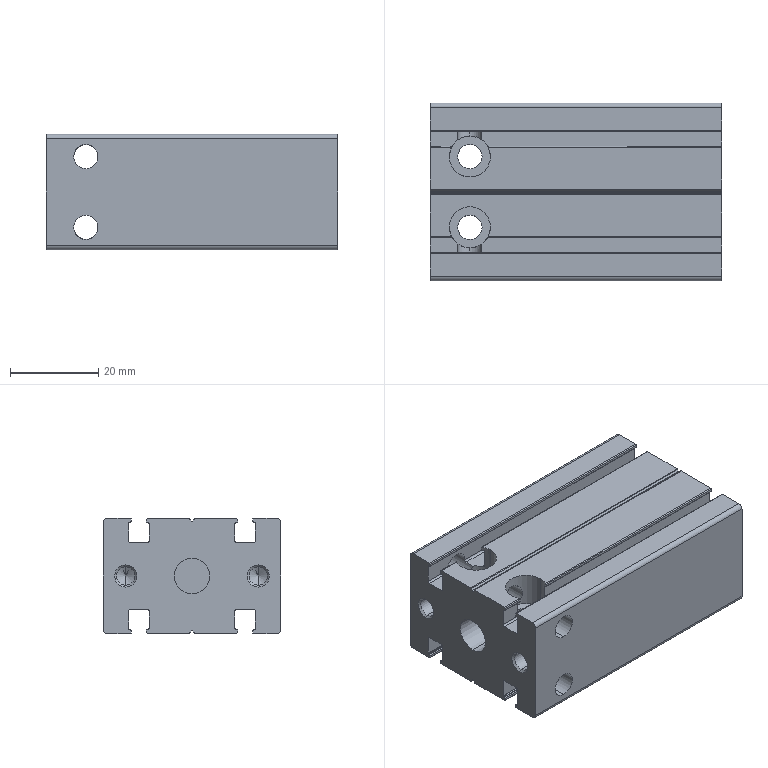Part | STEP file | 1 solid | 209 faces | box 66 x 40.2 x 26.2 mm | volume 46950 mm3 | cylinder 117 | plane 72 | cone 20 | commonest cylinder face diameters 0.4 x43 0.8 x16 5.5 x16 4.134 x12 9.3 x8 3 x6